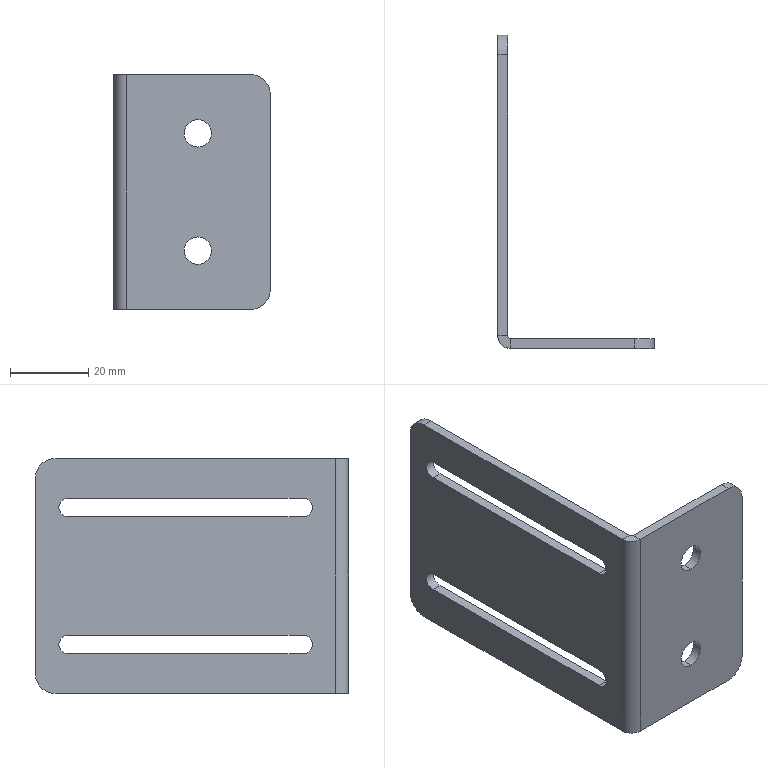Part | SolidWorks | features HoleWzd 2, BreakCorner 1, FlatPattern 1, SMBaseFlange 1, SheetMetal 1 | 1 solid | 30 faces | box 40 x 80 x 60 mm | volume 15721 mm3 | plane 16 | cylinder 14 | commonest cylinder face diameters 4.8 x4 7 x4 10 x4 1.473 x1 6.473 x1
STEP:
#1=CARTESIAN_POINT('',(21.5,0.,11.5));
#2=VERTEX_POINT('',#1);
#3=CARTESIAN_POINT('',(21.5,0.,18.5));
#4=VERTEX_POINT('',#3);
#5=CARTESIAN_POINT('',(21.5,0.,15.));
#6=DIRECTION('',(0.,1.,0.));
#7=DIRECTION('',(0.,0.,1.));
#8=AXIS2_PLACEMENT_3D('',#5,#6,#7);
#9=CIRCLE('',#8,3.5);
#10=EDGE_CURVE('',#2,#4,#9,.T.);
#11=ORIENTED_EDGE('',*,*,#10,.F.);
#12=CARTESIAN_POINT('',(21.5,2.5,11.5));
#13=VERTEX_POINT('',#12);
#14=CARTESIAN_POINT('',(21.5,2.5,11.5));
#15=DIRECTION('',(0.,1.,0.));
#16=VECTOR('',#15,1000.);
#17=LINE('',#14,#16);
#18=EDGE_CURVE('',#2,#13,#17,.T.);
#19=ORIENTED_EDGE('',*,*,#18,.T.);
#20=CARTESIAN_POINT('',(21.5,2.5,18.5));
#21=VERTEX_POINT('',#20);
#22=CARTESIAN_POINT('',(21.5,2.5,15.));
#23=DIRECTION('',(0.,1.,0.));
#24=DIRECTION('',(0.,0.,1.));
#25=AXIS2_PLACEMENT_3D('',#22,#23,#24);
#26=CIRCLE('',#25,3.5);
#27=EDGE_CURVE('',#13,#21,#26,.T.);
#28=ORIENTED_EDGE('',*,*,#27,.T.);
#29=CARTESIAN_POINT('',(21.5,2.5,18.5));
#30=DIRECTION('',(0.,1.,0.));
#31=VECTOR('',#30,1000.);
#32=LINE('',#29,#31);
#33=EDGE_CURVE('',#4,#21,#32,.T.);
#34=ORIENTED_EDGE('',*,*,#33,.F.);
#35=EDGE_LOOP('',(#11,#19,#28,#34));
#36=FACE_OUTER_BOUND('',#35,.T.);
#37=CARTESIAN_POINT('',(21.5,2.5,15.));
#38=DIRECTION('',(0.,1.,0.));
#39=DIRECTION('',(0.,0.,1.));
#40=AXIS2_PLACEMENT_3D('',#37,#38,#39);
#41=CYLINDRICAL_SURFACE('',#40,3.5);
#42=ADVANCED_FACE('',(#36),#41,.F.);
#43=CARTESIAN_POINT('',(21.5,0.,41.5));
#44=VERTEX_POINT('',#43);
#45=CARTESIAN_POINT('',(21.5,0.,48.5));
#46=VERTEX_POINT('',#45);
#47=CARTESIAN_POINT('',(21.5,0.,45.));
#48=DIRECTION('',(0.,1.,0.));
#49=DIRECTION('',(0.,0.,1.));
#50=AXIS2_PLACEMENT_3D('',#47,#48,#49);
#51=CIRCLE('',#50,3.5);
#52=EDGE_CURVE('',#44,#46,#51,.T.);
#53=ORIENTED_EDGE('',*,*,#52,.F.);
#54=CARTESIAN_POINT('',(21.5,2.5,41.5));
#55=VERTEX_POINT('',#54);
#56=CARTESIAN_POINT('',(21.5,2.5,41.5));
#57=DIRECTION('',(0.,1.,0.));
#58=VECTOR('',#57,1000.);
#59=LINE('',#56,#58);
#60=EDGE_CURVE('',#44,#55,#59,.T.);
#61=ORIENTED_EDGE('',*,*,#60,.T.);
#62=CARTESIAN_POINT('',(21.5,2.5,48.5));
#63=VERTEX_POINT('',#62);
#64=CARTESIAN_POINT('',(21.5,2.5,45.));
#65=DIRECTION('',(0.,1.,0.));
#66=DIRECTION('',(0.,0.,1.));
#67=AXIS2_PLACEMENT_3D('',#64,#65,#66);
#68=CIRCLE('',#67,3.5);
#69=EDGE_CURVE('',#55,#63,#68,.T.);
#70=ORIENTED_EDGE('',*,*,#69,.T.);
#71=CARTESIAN_POINT('',(21.5,2.5,48.5));
#72=DIRECTION('',(0.,1.,0.));
#73=VECTOR('',#72,1000.);
#74=LINE('',#71,#73);
#75=EDGE_CURVE('',#46,#63,#74,.T.);
#76=ORIENTED_EDGE('',*,*,#75,.F.);
#77=EDGE_LOOP('',(#53,#61,#70,#76));
#78=FACE_OUTER_BOUND('',#77,.T.);
#79=CARTESIAN_POINT('',(21.5,2.5,45.));
#80=DIRECTION('',(0.,1.,0.));
#81=DIRECTION('',(0.,0.,1.));
#82=AXIS2_PLACEMENT_3D('',#79,#80,#81);
#83=CYLINDRICAL_SURFACE('',#82,3.5);
#84=ADVANCED_FACE('',(#78),#83,.F.);
#85=CARTESIAN_POINT('',(0.,3.237,60.));
#86=VERTEX_POINT('',#85);
#87=CARTESIAN_POINT('',(2.5,3.237,60.));
#88=VERTEX_POINT('',#87);
#89=CARTESIAN_POINT('',(0.,3.237,60.));
#90=DIRECTION('',(1.,0.,0.));
#91=VECTOR('',#90,1000.);
#92=LINE('',#89,#91);
#93=EDGE_CURVE('',#86,#88,#92,.T.);
#94=ORIENTED_EDGE('',*,*,#93,.F.);
#95=CARTESIAN_POINT('',(3.237,0.,60.));
#96=VERTEX_POINT('',#95);
#97=CARTESIAN_POINT('',(3.237,3.237,60.));
#98=DIRECTION('',(0.,0.,-1.));
#99=DIRECTION('',(1.,0.,0.));
#100=AXIS2_PLACEMENT_3D('',#97,#98,#99);
#101=CIRCLE('',#100,3.237);
#102=EDGE_CURVE('',#96,#86,#101,.T.);
#103=ORIENTED_EDGE('',*,*,#102,.F.);
#104=CARTESIAN_POINT('',(3.237,2.5,60.));
#105=VERTEX_POINT('',#104);
#106=CARTESIAN_POINT('',(3.237,2.5,60.));
#107=DIRECTION('',(0.,-1.,0.));
#108=VECTOR('',#107,1000.);
#109=LINE('',#106,#108);
#110=EDGE_CURVE('',#105,#96,#109,.T.);
#111=ORIENTED_EDGE('',*,*,#110,.F.);
#112=CARTESIAN_POINT('',(3.237,3.237,60.));
#113=DIRECTION('',(0.,0.,-1.));
#114=DIRECTION('',(1.,0.,0.));
#115=AXIS2_PLACEMENT_3D('',#112,#113,#114);
#116=CIRCLE('',#115,0.7366);
#117=EDGE_CURVE('',#105,#88,#116,.T.);
#118=ORIENTED_EDGE('',*,*,#117,.T.);
#119=EDGE_LOOP('',(#94,#103,#111,#118));
#120=FACE_OUTER_BOUND('',#119,.T.);
#121=CARTESIAN_POINT('',(0.,3.237,60.));
#122=DIRECTION('',(0.,0.,1.));
#123=DIRECTION('',(1.,0.,0.));
#124=AXIS2_PLACEMENT_3D('',#121,#122,#123);
#125=PLANE('',#124);
#126=ADVANCED_FACE('',(#120),#125,.T.);
#127=CARTESIAN_POINT('',(2.5,75.,60.));
#128=VERTEX_POINT('',#127);
#129=CARTESIAN_POINT('',(2.5,0.,60.));
#130=DIRECTION('',(0.,1.,0.));
#131=VECTOR('',#130,1000.);
#132=LINE('',#129,#131);
#133=EDGE_CURVE('',#88,#128,#132,.T.);
#134=ORIENTED_EDGE('',*,*,#133,.T.);
#135=CARTESIAN_POINT('',(0.,75.,60.));
#136=VERTEX_POINT('',#135);
#137=CARTESIAN_POINT('',(3.237,75.,60.));
#138=DIRECTION('',(-1.,0.,0.));
#139=VECTOR('',#138,1000.);
#140=LINE('',#137,#139);
#141=EDGE_CURVE('',#128,#136,#140,.T.);
#142=ORIENTED_EDGE('',*,*,#141,.T.);
#143=CARTESIAN_POINT('',(0.,0.,60.));
#144=DIRECTION('',(0.,1.,0.));
#145=VECTOR('',#144,1000.);
#146=LINE('',#143,#145);
#147=EDGE_CURVE('',#86,#136,#146,.T.);
#148=ORIENTED_EDGE('',*,*,#147,.F.);
#149=ORIENTED_EDGE('',*,*,#93,.T.);
#150=EDGE_LOOP('',(#134,#142,#148,#149));
#151=FACE_OUTER_BOUND('',#150,.T.);
#152=CARTESIAN_POINT('',(3.237,2.5,60.));
#153=DIRECTION('',(0.,0.,1.));
#154=DIRECTION('',(1.,0.,0.));
#155=AXIS2_PLACEMENT_3D('',#152,#153,#154);
#156=PLANE('',#155);
#157=ADVANCED_FACE('',(#151),#156,.T.);
#158=CARTESIAN_POINT('',(3.237,0.,0.));
#159=VERTEX_POINT('',#158);
#160=CARTESIAN_POINT('',(3.237,2.5,0.));
#161=VERTEX_POINT('',#160);
#162=CARTESIAN_POINT('',(3.237,0.,0.));
#163=DIRECTION('',(0.,1.,0.));
#164=VECTOR('',#163,1000.);
#165=LINE('',#162,#164);
#166=EDGE_CURVE('',#159,#161,#165,.T.);
#167=ORIENTED_EDGE('',*,*,#166,.F.);
#168=CARTESIAN_POINT('',(0.,3.237,0.));
#169=VERTEX_POINT('',#168);
#170=CARTESIAN_POINT('',(3.237,3.237,0.));
#171=DIRECTION('',(0.,0.,-1.));
#172=DIRECTION('',(1.,0.,0.));
#173=AXIS2_PLACEMENT_3D('',#170,#171,#172);
#174=CIRCLE('',#173,3.237);
#175=EDGE_CURVE('',#159,#169,#174,.T.);
#176=ORIENTED_EDGE('',*,*,#175,.T.);
#177=CARTESIAN_POINT('',(2.5,3.237,0.));
#178=VERTEX_POINT('',#177);
#179=CARTESIAN_POINT('',(2.5,3.237,0.));
#180=DIRECTION('',(-1.,0.,0.));
#181=VECTOR('',#180,1000.);
#182=LINE('',#179,#181);
#183=EDGE_CURVE('',#178,#169,#182,.T.);
#184=ORIENTED_EDGE('',*,*,#183,.F.);
#185=CARTESIAN_POINT('',(3.237,3.237,0.));
#186=DIRECTION('',(0.,0.,-1.));
#187=DIRECTION('',(1.,0.,0.));
#188=AXIS2_PLACEMENT_3D('',#185,#186,#187);
#189=CIRCLE('',#188,0.7366);
#190=EDGE_CURVE('',#161,#178,#189,.T.);
#191=ORIENTED_EDGE('',*,*,#190,.F.);
#192=EDGE_LOOP('',(#167,#176,#184,#191));
#193=FACE_OUTER_BOUND('',#192,.T.);
#194=CARTESIAN_POINT('',(3.237,0.,0.));
#195=DIRECTION('',(0.,0.,-1.));
#196=DIRECTION('',(-1.,0.,0.));
#197=AXIS2_PLACEMENT_3D('',#194,#195,#196);
#198=PLANE('',#197);
#199=ADVANCED_FACE('',(#193),#198,.T.);
#200=CARTESIAN_POINT('',(35.,2.5,0.));
#201=VERTEX_POINT('',#200);
#202=CARTESIAN_POINT('',(0.,2.5,0.));
#203=DIRECTION('',(-1.,0.,0.));
#204=VECTOR('',#203,1000.);
#205=LINE('',#202,#204);
#206=EDGE_CURVE('',#201,#161,#205,.T.);
#207=ORIENTED_EDGE('',*,*,#206,.F.);
#208=CARTESIAN_POINT('',(35.,0.,0.));
#209=VERTEX_POINT('',#208);
#210=CARTESIAN_POINT('',(35.,3.237,0.));
#211=DIRECTION('',(0.,-1.,0.));
#212=VECTOR('',#211,1000.);
#213=LINE('',#210,#212);
#214=EDGE_CURVE('',#201,#209,#213,.T.);
#215=ORIENTED_EDGE('',*,*,#214,.T.);
#216=CARTESIAN_POINT('',(0.,0.,0.));
#217=DIRECTION('',(-1.,0.,0.));
#218=VECTOR('',#217,1000.);
#219=LINE('',#216,#218);
#220=EDGE_CURVE('',#209,#159,#219,.T.);
#221=ORIENTED_EDGE('',*,*,#220,.T.);
#222=ORIENTED_EDGE('',*,*,#166,.T.);
#223=EDGE_LOOP('',(#207,#215,#221,#222));
#224=FACE_OUTER_BOUND('',#223,.T.);
#225=CARTESIAN_POINT('',(2.5,3.237,0.));
#226=DIRECTION('',(0.,0.,-1.));
#227=DIRECTION('',(-1.,0.,0.));
#228=AXIS2_PLACEMENT_3D('',#225,#226,#227);
#229=PLANE('',#228);
#230=ADVANCED_FACE('',(#224),#229,.T.);
#231=CARTESIAN_POINT('',(2.5,11.618,49.9));
#232=VERTEX_POINT('',#231);
#233=CARTESIAN_POINT('',(2.5,11.618,45.1));
#234=VERTEX_POINT('',#233);
#235=CARTESIAN_POINT('',(2.5,11.618,47.5));
#236=DIRECTION('',(1.,0.,0.));
#237=DIRECTION('',(0.,0.,-1.));
#238=AXIS2_PLACEMENT_3D('',#235,#236,#237);
#239=CIRCLE('',#238,2.4);
#240=EDGE_CURVE('',#232,#234,#239,.T.);
#241=ORIENTED_EDGE('',*,*,#240,.F.);
#242=CARTESIAN_POINT('',(2.5,71.618,49.9));
#243=VERTEX_POINT('',#242);
#244=CARTESIAN_POINT('',(2.5,11.618,49.9));
#245=DIRECTION('',(0.,1.,0.));
#246=VECTOR('',#245,1000.);
#247=LINE('',#244,#246);
#248=EDGE_CURVE('',#232,#243,#247,.T.);
#249=ORIENTED_EDGE('',*,*,#248,.T.);
#250=CARTESIAN_POINT('',(2.5,71.618,45.1));
#251=VERTEX_POINT('',#250);
#252=CARTESIAN_POINT('',(2.5,71.618,47.5));
#253=DIRECTION('',(1.,0.,0.));
#254=DIRECTION('',(0.,0.,-1.));
#255=AXIS2_PLACEMENT_3D('',#252,#253,#254);
#256=CIRCLE('',#255,2.4);
#257=EDGE_CURVE('',#251,#243,#256,.T.);
#258=ORIENTED_EDGE('',*,*,#257,.F.);
#259=CARTESIAN_POINT('',(2.5,11.618,45.1));
#260=DIRECTION('',(0.,1.,0.));
#261=VECTOR('',#260,1000.);
#262=LINE('',#259,#261);
#263=EDGE_CURVE('',#234,#251,#262,.T.);
#264=ORIENTED_EDGE('',*,*,#263,.F.);
#265=EDGE_LOOP('',(#241,#249,#258,#264));
#266=FACE_BOUND('',#265,.T.);
#267=CARTESIAN_POINT('',(2.5,11.618,14.9));
#268=VERTEX_POINT('',#267);
#269=CARTESIAN_POINT('',(2.5,11.618,10.1));
#270=VERTEX_POINT('',#269);
#271=CARTESIAN_POINT('',(2.5,11.618,12.5));
#272=DIRECTION('',(1.,0.,0.));
#273=DIRECTION('',(0.,0.,-1.));
#274=AXIS2_PLACEMENT_3D('',#271,#272,#273);
#275=CIRCLE('',#274,2.4);
#276=EDGE_CURVE('',#268,#270,#275,.T.);
#277=ORIENTED_EDGE('',*,*,#276,.F.);
#278=CARTESIAN_POINT('',(2.5,71.618,14.9));
#279=VERTEX_POINT('',#278);
#280=CARTESIAN_POINT('',(2.5,11.618,14.9));
#281=DIRECTION('',(0.,1.,0.));
#282=VECTOR('',#281,1000.);
#283=LINE('',#280,#282);
#284=EDGE_CURVE('',#268,#279,#283,.T.);
#285=ORIENTED_EDGE('',*,*,#284,.T.);
#286=CARTESIAN_POINT('',(2.5,71.618,10.1));
#287=VERTEX_POINT('',#286);
#288=CARTESIAN_POINT('',(2.5,71.618,12.5));
#289=DIRECTION('',(1.,0.,0.));
#290=DIRECTION('',(0.,0.,-1.));
#291=AXIS2_PLACEMENT_3D('',#288,#289,#290);
#292=CIRCLE('',#291,2.4);
#293=EDGE_CURVE('',#287,#279,#292,.T.);
#294=ORIENTED_EDGE('',*,*,#293,.F.);
#295=CARTESIAN_POINT('',(2.5,11.618,10.1));
#296=DIRECTION('',(0.,1.,0.));
#297=VECTOR('',#296,1000.);
#298=LINE('',#295,#297);
#299=EDGE_CURVE('',#270,#287,#298,.T.);
#300=ORIENTED_EDGE('',*,*,#299,.F.);
#301=EDGE_LOOP('',(#277,#285,#294,#300));
#302=FACE_BOUND('',#301,.T.);
#303=CARTESIAN_POINT('',(2.5,80.,55.));
#304=VERTEX_POINT('',#303);
#305=CARTESIAN_POINT('',(2.5,80.,5.));
#306=VERTEX_POINT('',#305);
#307=CARTESIAN_POINT('',(2.5,80.,60.));
#308=DIRECTION('',(0.,0.,-1.));
#309=VECTOR('',#308,1000.);
#310=LINE('',#307,#309);
#311=EDGE_CURVE('',#304,#306,#310,.T.);
#312=ORIENTED_EDGE('',*,*,#311,.F.);
#313=CARTESIAN_POINT('',(2.5,75.,55.));
#314=DIRECTION('',(1.,0.,0.));
#315=DIRECTION('',(0.,0.,1.));
#316=AXIS2_PLACEMENT_3D('',#313,#314,#315);
#317=CIRCLE('',#316,5.);
#318=EDGE_CURVE('',#304,#128,#317,.T.);
#319=ORIENTED_EDGE('',*,*,#318,.T.);
#320=ORIENTED_EDGE('',*,*,#133,.F.);
#321=CARTESIAN_POINT('',(2.5,3.237,60.));
#322=DIRECTION('',(0.,0.,-1.));
#323=VECTOR('',#322,1000.);
#324=LINE('',#321,#323);
#325=EDGE_CURVE('',#88,#178,#324,.T.);
#326=ORIENTED_EDGE('',*,*,#325,.T.);
#327=CARTESIAN_POINT('',(2.5,75.,0.));
#328=VERTEX_POINT('',#327);
#329=CARTESIAN_POINT('',(2.5,0.,0.));
#330=DIRECTION('',(0.,1.,0.));
#331=VECTOR('',#330,1000.);
#332=LINE('',#329,#331);
#333=EDGE_CURVE('',#178,#328,#332,.T.);
#334=ORIENTED_EDGE('',*,*,#333,.T.);
#335=CARTESIAN_POINT('',(2.5,75.,5.));
#336=DIRECTION('',(1.,0.,0.));
#337=DIRECTION('',(0.,0.,1.));
#338=AXIS2_PLACEMENT_3D('',#335,#336,#337);
#339=CIRCLE('',#338,5.);
#340=EDGE_CURVE('',#328,#306,#339,.T.);
#341=ORIENTED_EDGE('',*,*,#340,.T.);
#342=EDGE_LOOP('',(#312,#319,#320,#326,#334,#341));
#343=FACE_OUTER_BOUND('',#342,.T.);
#344=CARTESIAN_POINT('',(2.5,0.,60.));
#345=DIRECTION('',(-1.,0.,0.));
#346=DIRECTION('',(0.,0.,1.));
#347=AXIS2_PLACEMENT_3D('',#344,#345,#346);
#348=PLANE('',#347);
#349=ADVANCED_FACE('',(#266,#302,#343),#348,.F.);
#350=CARTESIAN_POINT('',(0.,80.,55.));
#351=VERTEX_POINT('',#350);
#352=CARTESIAN_POINT('',(0.,80.,5.));
#353=VERTEX_POINT('',#352);
#354=CARTESIAN_POINT('',(0.,80.,60.));
#355=DIRECTION('',(0.,0.,-1.));
#356=VECTOR('',#355,1000.);
#357=LINE('',#354,#356);
#358=EDGE_CURVE('',#351,#353,#357,.T.);
#359=ORIENTED_EDGE('',*,*,#358,.F.);
#360=CARTESIAN_POINT('',(0.,80.,55.));
#361=DIRECTION('',(1.,0.,0.));
#362=VECTOR('',#361,1000.);
#363=LINE('',#360,#362);
#364=EDGE_CURVE('',#351,#304,#363,.T.);
#365=ORIENTED_EDGE('',*,*,#364,.T.);
#366=ORIENTED_EDGE('',*,*,#311,.T.);
#367=CARTESIAN_POINT('',(0.,80.,5.));
#368=DIRECTION('',(-1.,0.,0.));
#369=VECTOR('',#368,1000.);
#370=LINE('',#367,#369);
#371=EDGE_CURVE('',#306,#353,#370,.T.);
#372=ORIENTED_EDGE('',*,*,#371,.T.);
#373=EDGE_LOOP('',(#359,#365,#366,#372));
#374=FACE_OUTER_BOUND('',#373,.T.);
#375=CARTESIAN_POINT('',(0.,80.,60.));
#376=DIRECTION('',(0.,1.,0.));
#377=DIRECTION('',(0.,0.,1.));
#378=AXIS2_PLACEMENT_3D('',#375,#376,#377);
#379=PLANE('',#378);
#380=ADVANCED_FACE('',(#374),#379,.T.);
#381=CARTESIAN_POINT('',(0.,11.618,49.9));
#382=VERTEX_POINT('',#381);
#383=CARTESIAN_POINT('',(0.,71.618,49.9));
#384=VERTEX_POINT('',#383);
#385=CARTESIAN_POINT('',(0.,11.618,49.9));
#386=DIRECTION('',(0.,1.,0.));
#387=VECTOR('',#386,1000.);
#388=LINE('',#385,#387);
#389=EDGE_CURVE('',#382,#384,#388,.T.);
#390=ORIENTED_EDGE('',*,*,#389,.F.);
#391=CARTESIAN_POINT('',(0.,11.618,45.1));
#392=VERTEX_POINT('',#391);
#393=CARTESIAN_POINT('',(0.,11.618,47.5));
#394=DIRECTION('',(1.,0.,0.));
#395=DIRECTION('',(0.,0.,-1.));
#396=AXIS2_PLACEMENT_3D('',#393,#394,#395);
#397=CIRCLE('',#396,2.4);
#398=EDGE_CURVE('',#382,#392,#397,.T.);
#399=ORIENTED_EDGE('',*,*,#398,.T.);
#400=CARTESIAN_POINT('',(0.,71.618,45.1));
#401=VERTEX_POINT('',#400);
#402=CARTESIAN_POINT('',(0.,11.618,45.1));
#403=DIRECTION('',(0.,1.,0.));
#404=VECTOR('',#403,1000.);
#405=LINE('',#402,#404);
#406=EDGE_CURVE('',#392,#401,#405,.T.);
#407=ORIENTED_EDGE('',*,*,#406,.T.);
#408=CARTESIAN_POINT('',(0.,71.618,47.5));
#409=DIRECTION('',(1.,0.,0.));
#410=DIRECTION('',(0.,0.,-1.));
#411=AXIS2_PLACEMENT_3D('',#408,#409,#410);
#412=CIRCLE('',#411,2.4);
#413=EDGE_CURVE('',#401,#384,#412,.T.);
#414=ORIENTED_EDGE('',*,*,#413,.T.);
#415=EDGE_LOOP('',(#390,#399,#407,#414));
#416=FACE_BOUND('',#415,.T.);
#417=CARTESIAN_POINT('',(0.,11.618,14.9));
#418=VERTEX_POINT('',#417);
#419=CARTESIAN_POINT('',(0.,71.618,14.9));
#420=VERTEX_POINT('',#419);
#421=CARTESIAN_POINT('',(0.,11.618,14.9));
#422=DIRECTION('',(0.,1.,0.));
#423=VECTOR('',#422,1000.);
#424=LINE('',#421,#423);
#425=EDGE_CURVE('',#418,#420,#424,.T.);
#426=ORIENTED_EDGE('',*,*,#425,.F.);
#427=CARTESIAN_POINT('',(0.,11.618,10.1));
#428=VERTEX_POINT('',#427);
#429=CARTESIAN_POINT('',(0.,11.618,12.5));
#430=DIRECTION('',(1.,0.,0.));
#431=DIRECTION('',(0.,0.,-1.));
#432=AXIS2_PLACEMENT_3D('',#429,#430,#431);
#433=CIRCLE('',#432,2.4);
#434=EDGE_CURVE('',#418,#428,#433,.T.);
#435=ORIENTED_EDGE('',*,*,#434,.T.);
#436=CARTESIAN_POINT('',(0.,71.618,10.1));
#437=VERTEX_POINT('',#436);
#438=CARTESIAN_POINT('',(0.,11.618,10.1));
#439=DIRECTION('',(0.,1.,0.));
#440=VECTOR('',#439,1000.);
#441=LINE('',#438,#440);
#442=EDGE_CURVE('',#428,#437,#441,.T.);
#443=ORIENTED_EDGE('',*,*,#442,.T.);
#444=CARTESIAN_POINT('',(0.,71.618,12.5));
#445=DIRECTION('',(1.,0.,0.));
#446=DIRECTION('',(0.,0.,-1.));
#447=AXIS2_PLACEMENT_3D('',#444,#445,#446);
#448=CIRCLE('',#447,2.4);
#449=EDGE_CURVE('',#437,#420,#448,.T.);
#450=ORIENTED_EDGE('',*,*,#449,.T.);
#451=EDGE_LOOP('',(#426,#435,#443,#450));
#452=FACE_BOUND('',#451,.T.);
#453=ORIENTED_EDGE('',*,*,#147,.T.);
#454=CARTESIAN_POINT('',(0.,75.,55.));
#455=DIRECTION('',(-1.,0.,0.));
#456=DIRECTION('',(0.,0.,1.));
#457=AXIS2_PLACEMENT_3D('',#454,#455,#456);
#458=CIRCLE('',#457,5.);
#459=EDGE_CURVE('',#136,#351,#458,.T.);
#460=ORIENTED_EDGE('',*,*,#459,.T.);
#461=ORIENTED_EDGE('',*,*,#358,.T.);
#462=CARTESIAN_POINT('',(0.,75.,0.));
#463=VERTEX_POINT('',#462);
#464=CARTESIAN_POINT('',(0.,75.,5.));
#465=DIRECTION('',(-1.,0.,0.));
#466=DIRECTION('',(0.,0.,1.));
#467=AXIS2_PLACEMENT_3D('',#464,#465,#466);
#468=CIRCLE('',#467,5.);
#469=EDGE_CURVE('',#353,#463,#468,.T.);
#470=ORIENTED_EDGE('',*,*,#469,.T.);
#471=CARTESIAN_POINT('',(0.,0.,0.));
#472=DIRECTION('',(0.,1.,0.));
#473=VECTOR('',#472,1000.);
#474=LINE('',#471,#473);
#475=EDGE_CURVE('',#169,#463,#474,.T.);
#476=ORIENTED_EDGE('',*,*,#475,.F.);
#477=CARTESIAN_POINT('',(0.,3.237,60.));
#478=DIRECTION('',(0.,0.,-1.));
#479=VECTOR('',#478,1000.);
#480=LINE('',#477,#479);
#481=EDGE_CURVE('',#86,#169,#480,.T.);
#482=ORIENTED_EDGE('',*,*,#481,.F.);
#483=EDGE_LOOP('',(#453,#460,#461,#470,#476,#482));
#484=FACE_OUTER_BOUND('',#483,.T.);
#485=CARTESIAN_POINT('',(0.,0.,60.));
#486=DIRECTION('',(-1.,0.,0.));
#487=DIRECTION('',(0.,0.,1.));
#488=AXIS2_PLACEMENT_3D('',#485,#486,#487);
#489=PLANE('',#488);
#490=ADVANCED_FACE('',(#416,#452,#484),#489,.T.);
#491=ORIENTED_EDGE('',*,*,#175,.F.);
#492=CARTESIAN_POINT('',(3.237,0.,60.));
#493=DIRECTION('',(0.,0.,-1.));
#494=VECTOR('',#493,1000.);
#495=LINE('',#492,#494);
#496=EDGE_CURVE('',#96,#159,#495,.T.);
#497=ORIENTED_EDGE('',*,*,#496,.F.);
#498=ORIENTED_EDGE('',*,*,#102,.T.);
#499=ORIENTED_EDGE('',*,*,#481,.T.);
#500=EDGE_LOOP('',(#491,#497,#498,#499));
#501=FACE_OUTER_BOUND('',#500,.T.);
#502=CARTESIAN_POINT('',(3.237,3.237,60.));
#503=DIRECTION('',(0.,0.,-1.));
#504=DIRECTION('',(-1.,0.,0.));
#505=AXIS2_PLACEMENT_3D('',#502,#503,#504);
#506=CYLINDRICAL_SURFACE('',#505,3.237);
#507=ADVANCED_FACE('',(#501),#506,.T.);
#508=CARTESIAN_POINT('',(21.5,0.,15.));
#509=DIRECTION('',(0.,1.,0.));
#510=DIRECTION('',(0.,0.,1.));
#511=AXIS2_PLACEMENT_3D('',#508,#509,#510);
#512=CIRCLE('',#511,3.5);
#513=EDGE_CURVE('',#4,#2,#512,.T.);
#514=ORIENTED_EDGE('',*,*,#513,.T.);
#515=ORIENTED_EDGE('',*,*,#10,.T.);
#516=EDGE_LOOP('',(#514,#515));
#517=FACE_BOUND('',#516,.T.);
#518=CARTESIAN_POINT('',(21.5,0.,45.));
#519=DIRECTION('',(0.,1.,0.));
#520=DIRECTION('',(0.,0.,1.));
#521=AXIS2_PLACEMENT_3D('',#518,#519,#520);
#522=CIRCLE('',#521,3.5);
#523=EDGE_CURVE('',#46,#44,#522,.T.);
#524=ORIENTED_EDGE('',*,*,#523,.T.);
#525=ORIENTED_EDGE('',*,*,#52,.T.);
#526=EDGE_LOOP('',(#524,#525));
#527=FACE_BOUND('',#526,.T.);
#528=CARTESIAN_POINT('',(40.,0.,55.));
#529=VERTEX_POINT('',#528);
#530=CARTESIAN_POINT('',(40.,0.,5.));
#531=VERTEX_POINT('',#530);
#532=CARTESIAN_POINT('',(40.,0.,60.));
#533=DIRECTION('',(0.,0.,-1.));
#534=VECTOR('',#533,1000.);
#535=LINE('',#532,#534);
#536=EDGE_CURVE('',#529,#531,#535,.T.);
#537=ORIENTED_EDGE('',*,*,#536,.F.);
#538=CARTESIAN_POINT('',(35.,0.,60.));
#539=VERTEX_POINT('',#538);
#540=CARTESIAN_POINT('',(35.,0.,55.));
#541=DIRECTION('',(0.,-1.,0.));
#542=DIRECTION('',(0.,0.,-1.));
#543=AXIS2_PLACEMENT_3D('',#540,#541,#542);
#544=CIRCLE('',#543,5.);
#545=EDGE_CURVE('',#529,#539,#544,.T.);
#546=ORIENTED_EDGE('',*,*,#545,.T.);
#547=CARTESIAN_POINT('',(0.,0.,60.));
#548=DIRECTION('',(-1.,0.,0.));
#549=VECTOR('',#548,1000.);
#550=LINE('',#547,#549);
#551=EDGE_CURVE('',#539,#96,#550,.T.);
#552=ORIENTED_EDGE('',*,*,#551,.T.);
#553=ORIENTED_EDGE('',*,*,#496,.T.);
#554=ORIENTED_EDGE('',*,*,#220,.F.);
#555=CARTESIAN_POINT('',(35.,0.,5.));
#556=DIRECTION('',(0.,-1.,0.));
#557=DIRECTION('',(0.,0.,-1.));
#558=AXIS2_PLACEMENT_3D('',#555,#556,#557);
#559=CIRCLE('',#558,5.);
#560=EDGE_CURVE('',#209,#531,#559,.T.);
#561=ORIENTED_EDGE('',*,*,#560,.T.);
#562=EDGE_LOOP('',(#537,#546,#552,#553,#554,#561));
#563=FACE_OUTER_BOUND('',#562,.T.);
#564=CARTESIAN_POINT('',(0.,0.,60.));
#565=DIRECTION('',(0.,-1.,0.));
#566=DIRECTION('',(0.,0.,-1.));
#567=AXIS2_PLACEMENT_3D('',#564,#565,#566);
#568=PLANE('',#567);
#569=ADVANCED_FACE('',(#517,#527,#563),#568,.T.);
#570=CARTESIAN_POINT('',(40.,2.5,55.));
#571=VERTEX_POINT('',#570);
#572=CARTESIAN_POINT('',(40.,2.5,5.));
#573=VERTEX_POINT('',#572);
#574=CARTESIAN_POINT('',(40.,2.5,60.));
#575=DIRECTION('',(0.,0.,-1.));
#576=VECTOR('',#575,1000.);
#577=LINE('',#574,#576);
#578=EDGE_CURVE('',#571,#573,#577,.T.);
#579=ORIENTED_EDGE('',*,*,#578,.F.);
#580=CARTESIAN_POINT('',(40.,2.5,55.));
#581=DIRECTION('',(0.,-1.,0.));
#582=VECTOR('',#581,1000.);
#583=LINE('',#580,#582);
#584=EDGE_CURVE('',#571,#529,#583,.T.);
#585=ORIENTED_EDGE('',*,*,#584,.T.);
#586=ORIENTED_EDGE('',*,*,#536,.T.);
#587=CARTESIAN_POINT('',(40.,2.5,5.));
#588=DIRECTION('',(0.,1.,0.));
#589=VECTOR('',#588,1000.);
#590=LINE('',#587,#589);
#591=EDGE_CURVE('',#531,#573,#590,.T.);
#592=ORIENTED_EDGE('',*,*,#591,.T.);
#593=EDGE_LOOP('',(#579,#585,#586,#592));
#594=FACE_OUTER_BOUND('',#593,.T.);
#595=CARTESIAN_POINT('',(40.,2.5,60.));
#596=DIRECTION('',(1.,0.,0.));
#597=DIRECTION('',(0.,0.,-1.));
#598=AXIS2_PLACEMENT_3D('',#595,#596,#597);
#599=PLANE('',#598);
#600=ADVANCED_FACE('',(#594),#599,.T.);
#601=CARTESIAN_POINT('',(21.5,2.5,15.));
#602=DIRECTION('',(0.,1.,0.));
#603=DIRECTION('',(0.,0.,1.));
#604=AXIS2_PLACEMENT_3D('',#601,#602,#603);
#605=CIRCLE('',#604,3.5);
#606=EDGE_CURVE('',#21,#13,#605,.T.);
#607=ORIENTED_EDGE('',*,*,#606,.F.);
#608=ORIENTED_EDGE('',*,*,#27,.F.);
#609=EDGE_LOOP('',(#607,#608));
#610=FACE_BOUND('',#609,.T.);
#611=CARTESIAN_POINT('',(21.5,2.5,45.));
#612=DIRECTION('',(0.,1.,0.));
#613=DIRECTION('',(0.,0.,1.));
#614=AXIS2_PLACEMENT_3D('',#611,#612,#613);
#615=CIRCLE('',#614,3.5);
#616=EDGE_CURVE('',#63,#55,#615,.T.);
#617=ORIENTED_EDGE('',*,*,#616,.F.);
#618=ORIENTED_EDGE('',*,*,#69,.F.);
#619=EDGE_LOOP('',(#617,#618));
#620=FACE_BOUND('',#619,.T.);
#621=CARTESIAN_POINT('',(35.,2.5,60.));
#622=VERTEX_POINT('',#621);
#623=CARTESIAN_POINT('',(0.,2.5,60.));
#624=DIRECTION('',(-1.,0.,0.));
#625=VECTOR('',#624,1000.);
#626=LINE('',#623,#625);
#627=EDGE_CURVE('',#622,#105,#626,.T.);
#628=ORIENTED_EDGE('',*,*,#627,.F.);
#629=CARTESIAN_POINT('',(35.,2.5,55.));
#630=DIRECTION('',(0.,1.,0.));
#631=DIRECTION('',(0.,0.,-1.));
#632=AXIS2_PLACEMENT_3D('',#629,#630,#631);
#633=CIRCLE('',#632,5.);
#634=EDGE_CURVE('',#622,#571,#633,.T.);
#635=ORIENTED_EDGE('',*,*,#634,.T.);
#636=ORIENTED_EDGE('',*,*,#578,.T.);
#637=CARTESIAN_POINT('',(35.,2.5,5.));
#638=DIRECTION('',(0.,1.,0.));
#639=DIRECTION('',(0.,0.,-1.));
#640=AXIS2_PLACEMENT_3D('',#637,#638,#639);
#641=CIRCLE('',#640,5.);
#642=EDGE_CURVE('',#573,#201,#641,.T.);
#643=ORIENTED_EDGE('',*,*,#642,.T.);
#644=ORIENTED_EDGE('',*,*,#206,.T.);
#645=CARTESIAN_POINT('',(3.237,2.5,60.));
#646=DIRECTION('',(0.,0.,-1.));
#647=VECTOR('',#646,1000.);
#648=LINE('',#645,#647);
#649=EDGE_CURVE('',#105,#161,#648,.T.);
#650=ORIENTED_EDGE('',*,*,#649,.F.);
#651=EDGE_LOOP('',(#628,#635,#636,#643,#644,#650));
#652=FACE_OUTER_BOUND('',#651,.T.);
#653=CARTESIAN_POINT('',(0.,2.5,60.));
#654=DIRECTION('',(0.,-1.,0.));
#655=DIRECTION('',(0.,0.,-1.));
#656=AXIS2_PLACEMENT_3D('',#653,#654,#655);
#657=PLANE('',#656);
#658=ADVANCED_FACE('',(#610,#620,#652),#657,.F.);
#659=ORIENTED_EDGE('',*,*,#190,.T.);
#660=ORIENTED_EDGE('',*,*,#325,.F.);
#661=ORIENTED_EDGE('',*,*,#117,.F.);
#662=ORIENTED_EDGE('',*,*,#649,.T.);
#663=EDGE_LOOP('',(#659,#660,#661,#662));
#664=FACE_OUTER_BOUND('',#663,.T.);
#665=CARTESIAN_POINT('',(3.237,3.237,60.));
#666=DIRECTION('',(0.,0.,-1.));
#667=DIRECTION('',(-1.,0.,0.));
#668=AXIS2_PLACEMENT_3D('',#665,#666,#667);
#669=CYLINDRICAL_SURFACE('',#668,0.7366);
#670=ADVANCED_FACE('',(#664),#669,.F.);
#671=ORIENTED_EDGE('',*,*,#551,.F.);
#672=CARTESIAN_POINT('',(35.,3.237,60.));
#673=DIRECTION('',(0.,1.,0.));
#674=VECTOR('',#673,1000.);
#675=LINE('',#672,#674);
#676=EDGE_CURVE('',#539,#622,#675,.T.);
#677=ORIENTED_EDGE('',*,*,#676,.T.);
#678=ORIENTED_EDGE('',*,*,#627,.T.);
#679=ORIENTED_EDGE('',*,*,#110,.T.);
#680=EDGE_LOOP('',(#671,#677,#678,#679));
#681=FACE_OUTER_BOUND('',#680,.T.);
#682=CARTESIAN_POINT('',(3.237,3.237,60.));
#683=DIRECTION('',(0.,0.,1.));
#684=DIRECTION('',(1.,0.,0.));
#685=AXIS2_PLACEMENT_3D('',#682,#683,#684);
#686=PLANE('',#685);
#687=ADVANCED_FACE('',(#681),#686,.T.);
#688=ORIENTED_EDGE('',*,*,#475,.T.);
#689=CARTESIAN_POINT('',(2.5,75.,0.));
#690=DIRECTION('',(1.,0.,0.));
#691=VECTOR('',#690,1000.);
#692=LINE('',#689,#691);
#693=EDGE_CURVE('',#463,#328,#692,.T.);
#694=ORIENTED_EDGE('',*,*,#693,.T.);
#695=ORIENTED_EDGE('',*,*,#333,.F.);
#696=ORIENTED_EDGE('',*,*,#183,.T.);
#697=EDGE_LOOP('',(#688,#694,#695,#696));
#698=FACE_OUTER_BOUND('',#697,.T.);
#699=CARTESIAN_POINT('',(3.237,3.237,0.));
#700=DIRECTION('',(0.,0.,1.));
#701=DIRECTION('',(1.,0.,0.));
#702=AXIS2_PLACEMENT_3D('',#699,#700,#701);
#703=PLANE('',#702);
#704=ADVANCED_FACE('',(#698),#703,.F.);
#705=ORIENTED_EDGE('',*,*,#449,.F.);
#706=CARTESIAN_POINT('',(2.5,71.618,10.1));
#707=DIRECTION('',(-1.,0.,0.));
#708=VECTOR('',#707,1000.);
#709=LINE('',#706,#708);
#710=EDGE_CURVE('',#287,#437,#709,.T.);
#711=ORIENTED_EDGE('',*,*,#710,.F.);
#712=ORIENTED_EDGE('',*,*,#293,.T.);
#713=CARTESIAN_POINT('',(2.5,71.618,14.9));
#714=DIRECTION('',(1.,0.,0.));
#715=VECTOR('',#714,1000.);
#716=LINE('',#713,#715);
#717=EDGE_CURVE('',#420,#279,#716,.T.);
#718=ORIENTED_EDGE('',*,*,#717,.F.);
#719=EDGE_LOOP('',(#705,#711,#712,#718));
#720=FACE_OUTER_BOUND('',#719,.T.);
#721=CARTESIAN_POINT('',(2.5,71.618,12.5));
#722=DIRECTION('',(1.,0.,0.));
#723=DIRECTION('',(0.,0.,-1.));
#724=AXIS2_PLACEMENT_3D('',#721,#722,#723);
#725=CYLINDRICAL_SURFACE('',#724,2.4);
#726=ADVANCED_FACE('',(#720),#725,.F.);
#727=ORIENTED_EDGE('',*,*,#276,.T.);
#728=CARTESIAN_POINT('',(2.5,11.618,10.1));
#729=DIRECTION('',(1.,0.,0.));
#730=VECTOR('',#729,1000.);
#731=LINE('',#728,#730);
#732=EDGE_CURVE('',#428,#270,#731,.T.);
#733=ORIENTED_EDGE('',*,*,#732,.F.);
#734=ORIENTED_EDGE('',*,*,#434,.F.);
#735=CARTESIAN_POINT('',(2.5,11.618,14.9));
#736=DIRECTION('',(-1.,0.,0.));
#737=VECTOR('',#736,1000.);
#738=LINE('',#735,#737);
#739=EDGE_CURVE('',#268,#418,#738,.T.);
#740=ORIENTED_EDGE('',*,*,#739,.F.);
#741=EDGE_LOOP('',(#727,#733,#734,#740));
#742=FACE_OUTER_BOUND('',#741,.T.);
#743=CARTESIAN_POINT('',(2.5,11.618,12.5));
#744=DIRECTION('',(1.,0.,0.));
#745=DIRECTION('',(0.,0.,-1.));
#746=AXIS2_PLACEMENT_3D('',#743,#744,#745);
#747=CYLINDRICAL_SURFACE('',#746,2.4);
#748=ADVANCED_FACE('',(#742),#747,.F.);
#749=ORIENTED_EDGE('',*,*,#717,.T.);
#750=ORIENTED_EDGE('',*,*,#284,.F.);
#751=ORIENTED_EDGE('',*,*,#739,.T.);
#752=ORIENTED_EDGE('',*,*,#425,.T.);
#753=EDGE_LOOP('',(#749,#750,#751,#752));
#754=FACE_OUTER_BOUND('',#753,.T.);
#755=CARTESIAN_POINT('',(2.5,11.618,14.9));
#756=DIRECTION('',(0.,0.,1.));
#757=DIRECTION('',(1.,0.,0.));
#758=AXIS2_PLACEMENT_3D('',#755,#756,#757);
#759=PLANE('',#758);
#760=ADVANCED_FACE('',(#754),#759,.F.);
#761=ORIENTED_EDGE('',*,*,#710,.T.);
#762=ORIENTED_EDGE('',*,*,#442,.F.);
#763=ORIENTED_EDGE('',*,*,#732,.T.);
#764=ORIENTED_EDGE('',*,*,#299,.T.);
#765=EDGE_LOOP('',(#761,#762,#763,#764));
#766=FACE_OUTER_BOUND('',#765,.T.);
#767=CARTESIAN_POINT('',(2.5,11.618,10.1));
#768=DIRECTION('',(0.,0.,-1.));
#769=DIRECTION('',(-1.,0.,0.));
#770=AXIS2_PLACEMENT_3D('',#767,#768,#769);
#771=PLANE('',#770);
#772=ADVANCED_FACE('',(#766),#771,.F.);
#773=ORIENTED_EDGE('',*,*,#413,.F.);
#774=CARTESIAN_POINT('',(2.5,71.618,45.1));
#775=DIRECTION('',(-1.,0.,0.));
#776=VECTOR('',#775,1000.);
#777=LINE('',#774,#776);
#778=EDGE_CURVE('',#251,#401,#777,.T.);
#779=ORIENTED_EDGE('',*,*,#778,.F.);
#780=ORIENTED_EDGE('',*,*,#257,.T.);
#781=CARTESIAN_POINT('',(2.5,71.618,49.9));
#782=DIRECTION('',(1.,0.,0.));
#783=VECTOR('',#782,1000.);
#784=LINE('',#781,#783);
#785=EDGE_CURVE('',#384,#243,#784,.T.);
#786=ORIENTED_EDGE('',*,*,#785,.F.);
#787=EDGE_LOOP('',(#773,#779,#780,#786));
#788=FACE_OUTER_BOUND('',#787,.T.);
#789=CARTESIAN_POINT('',(2.5,71.618,47.5));
#790=DIRECTION('',(1.,0.,0.));
#791=DIRECTION('',(0.,0.,-1.));
#792=AXIS2_PLACEMENT_3D('',#789,#790,#791);
#793=CYLINDRICAL_SURFACE('',#792,2.4);
#794=ADVANCED_FACE('',(#788),#793,.F.);
#795=ORIENTED_EDGE('',*,*,#240,.T.);
#796=CARTESIAN_POINT('',(2.5,11.618,45.1));
#797=DIRECTION('',(1.,0.,0.));
#798=VECTOR('',#797,1000.);
#799=LINE('',#796,#798);
#800=EDGE_CURVE('',#392,#234,#799,.T.);
#801=ORIENTED_EDGE('',*,*,#800,.F.);
#802=ORIENTED_EDGE('',*,*,#398,.F.);
#803=CARTESIAN_POINT('',(2.5,11.618,49.9));
#804=DIRECTION('',(-1.,0.,0.));
#805=VECTOR('',#804,1000.);
#806=LINE('',#803,#805);
#807=EDGE_CURVE('',#232,#382,#806,.T.);
#808=ORIENTED_EDGE('',*,*,#807,.F.);
#809=EDGE_LOOP('',(#795,#801,#802,#808));
#810=FACE_OUTER_BOUND('',#809,.T.);
#811=CARTESIAN_POINT('',(2.5,11.618,47.5));
#812=DIRECTION('',(1.,0.,0.));
#813=DIRECTION('',(0.,0.,-1.));
#814=AXIS2_PLACEMENT_3D('',#811,#812,#813);
#815=CYLINDRICAL_SURFACE('',#814,2.4);
#816=ADVANCED_FACE('',(#810),#815,.F.);
#817=ORIENTED_EDGE('',*,*,#785,.T.);
#818=ORIENTED_EDGE('',*,*,#248,.F.);
#819=ORIENTED_EDGE('',*,*,#807,.T.);
#820=ORIENTED_EDGE('',*,*,#389,.T.);
#821=EDGE_LOOP('',(#817,#818,#819,#820));
#822=FACE_OUTER_BOUND('',#821,.T.);
#823=CARTESIAN_POINT('',(2.5,11.618,49.9));
#824=DIRECTION('',(0.,0.,1.));
#825=DIRECTION('',(1.,0.,0.));
#826=AXIS2_PLACEMENT_3D('',#823,#824,#825);
#827=PLANE('',#826);
#828=ADVANCED_FACE('',(#822),#827,.F.);
#829=ORIENTED_EDGE('',*,*,#778,.T.);
#830=ORIENTED_EDGE('',*,*,#406,.F.);
#831=ORIENTED_EDGE('',*,*,#800,.T.);
#832=ORIENTED_EDGE('',*,*,#263,.T.);
#833=EDGE_LOOP('',(#829,#830,#831,#832));
#834=FACE_OUTER_BOUND('',#833,.T.);
#835=CARTESIAN_POINT('',(2.5,11.618,45.1));
#836=DIRECTION('',(0.,0.,-1.));
#837=DIRECTION('',(-1.,0.,0.));
#838=AXIS2_PLACEMENT_3D('',#835,#836,#837);
#839=PLANE('',#838);
#840=ADVANCED_FACE('',(#834),#839,.F.);
#841=ORIENTED_EDGE('',*,*,#60,.F.);
#842=ORIENTED_EDGE('',*,*,#523,.F.);
#843=ORIENTED_EDGE('',*,*,#75,.T.);
#844=ORIENTED_EDGE('',*,*,#616,.T.);
#845=EDGE_LOOP('',(#841,#842,#843,#844));
#846=FACE_OUTER_BOUND('',#845,.T.);
#847=CARTESIAN_POINT('',(21.5,2.5,45.));
#848=DIRECTION('',(0.,1.,0.));
#849=DIRECTION('',(0.,0.,1.));
#850=AXIS2_PLACEMENT_3D('',#847,#848,#849);
#851=CYLINDRICAL_SURFACE('',#850,3.5);
#852=ADVANCED_FACE('',(#846),#851,.F.);
#853=ORIENTED_EDGE('',*,*,#18,.F.);
#854=ORIENTED_EDGE('',*,*,#513,.F.);
#855=ORIENTED_EDGE('',*,*,#33,.T.);
#856=ORIENTED_EDGE('',*,*,#606,.T.);
#857=EDGE_LOOP('',(#853,#854,#855,#856));
#858=FACE_OUTER_BOUND('',#857,.T.);
#859=CARTESIAN_POINT('',(21.5,2.5,15.));
#860=DIRECTION('',(0.,1.,0.));
#861=DIRECTION('',(0.,0.,1.));
#862=AXIS2_PLACEMENT_3D('',#859,#860,#861);
#863=CYLINDRICAL_SURFACE('',#862,3.5);
#864=ADVANCED_FACE('',(#858),#863,.F.);
#865=ORIENTED_EDGE('',*,*,#634,.F.);
#866=ORIENTED_EDGE('',*,*,#676,.F.);
#867=ORIENTED_EDGE('',*,*,#545,.F.);
#868=ORIENTED_EDGE('',*,*,#584,.F.);
#869=EDGE_LOOP('',(#865,#866,#867,#868));
#870=FACE_OUTER_BOUND('',#869,.T.);
#871=CARTESIAN_POINT('',(35.,2.5,55.));
#872=DIRECTION('',(0.,-1.,0.));
#873=DIRECTION('',(0.,0.,-1.));
#874=AXIS2_PLACEMENT_3D('',#871,#872,#873);
#875=CYLINDRICAL_SURFACE('',#874,5.);
#876=ADVANCED_FACE('',(#870),#875,.T.);
#877=ORIENTED_EDGE('',*,*,#642,.F.);
#878=ORIENTED_EDGE('',*,*,#591,.F.);
#879=ORIENTED_EDGE('',*,*,#560,.F.);
#880=ORIENTED_EDGE('',*,*,#214,.F.);
#881=EDGE_LOOP('',(#877,#878,#879,#880));
#882=FACE_OUTER_BOUND('',#881,.T.);
#883=CARTESIAN_POINT('',(35.,3.237,5.));
#884=DIRECTION('',(0.,-1.,0.));
#885=DIRECTION('',(0.,0.,-1.));
#886=AXIS2_PLACEMENT_3D('',#883,#884,#885);
#887=CYLINDRICAL_SURFACE('',#886,5.);
#888=ADVANCED_FACE('',(#882),#887,.T.);
#889=ORIENTED_EDGE('',*,*,#459,.F.);
#890=ORIENTED_EDGE('',*,*,#141,.F.);
#891=ORIENTED_EDGE('',*,*,#318,.F.);
#892=ORIENTED_EDGE('',*,*,#364,.F.);
#893=EDGE_LOOP('',(#889,#890,#891,#892));
#894=FACE_OUTER_BOUND('',#893,.T.);
#895=CARTESIAN_POINT('',(0.,75.,55.));
#896=DIRECTION('',(1.,0.,0.));
#897=DIRECTION('',(0.,0.,-1.));
#898=AXIS2_PLACEMENT_3D('',#895,#896,#897);
#899=CYLINDRICAL_SURFACE('',#898,5.);
#900=ADVANCED_FACE('',(#894),#899,.T.);
#901=ORIENTED_EDGE('',*,*,#469,.F.);
#902=ORIENTED_EDGE('',*,*,#371,.F.);
#903=ORIENTED_EDGE('',*,*,#340,.F.);
#904=ORIENTED_EDGE('',*,*,#693,.F.);
#905=EDGE_LOOP('',(#901,#902,#903,#904));
#906=FACE_OUTER_BOUND('',#905,.T.);
#907=CARTESIAN_POINT('',(3.237,75.,5.));
#908=DIRECTION('',(-1.,0.,0.));
#909=DIRECTION('',(0.,0.,1.));
#910=AXIS2_PLACEMENT_3D('',#907,#908,#909);
#911=CYLINDRICAL_SURFACE('',#910,5.);
#912=ADVANCED_FACE('',(#906),#911,.T.);
#913=CLOSED_SHELL('',(#42,#84,#126,#157,#199,#230,#349,#380,#490,#507,#569,#600,#658,#670,#687,#704,#726,#748,#760,#772,#794,#816,#828,#840,#852,#864,#876,#888,#900,#912));
#914=MANIFOLD_SOLID_BREP('',#913);
#915=CARTESIAN_POINT('',(0.,0.,0.));
#916=DIRECTION('',(0.,0.,1.));
#917=DIRECTION('',(1.,0.,0.));
#918=AXIS2_PLACEMENT_3D('',#915,#916,#917);
#919=(LENGTH_UNIT()NAMED_UNIT(*)SI_UNIT(.MILLI.,.METRE.));
#920=UNCERTAINTY_MEASURE_WITH_UNIT(LENGTH_MEASURE(0.00001),#919,'','');
#921=(NAMED_UNIT(*)PLANE_ANGLE_UNIT()SI_UNIT($,.RADIAN.));
#922=(NAMED_UNIT(*)SI_UNIT($,.STERADIAN.)SOLID_ANGLE_UNIT());
#923=(GEOMETRIC_REPRESENTATION_CONTEXT(3)GLOBAL_UNCERTAINTY_ASSIGNED_CONTEXT((#920))GLOBAL_UNIT_ASSIGNED_CONTEXT((#919,#921,#922))REPRESENTATION_CONTEXT('',''));
#924=ADVANCED_BREP_SHAPE_REPRESENTATION('',(#914,#918),#923);